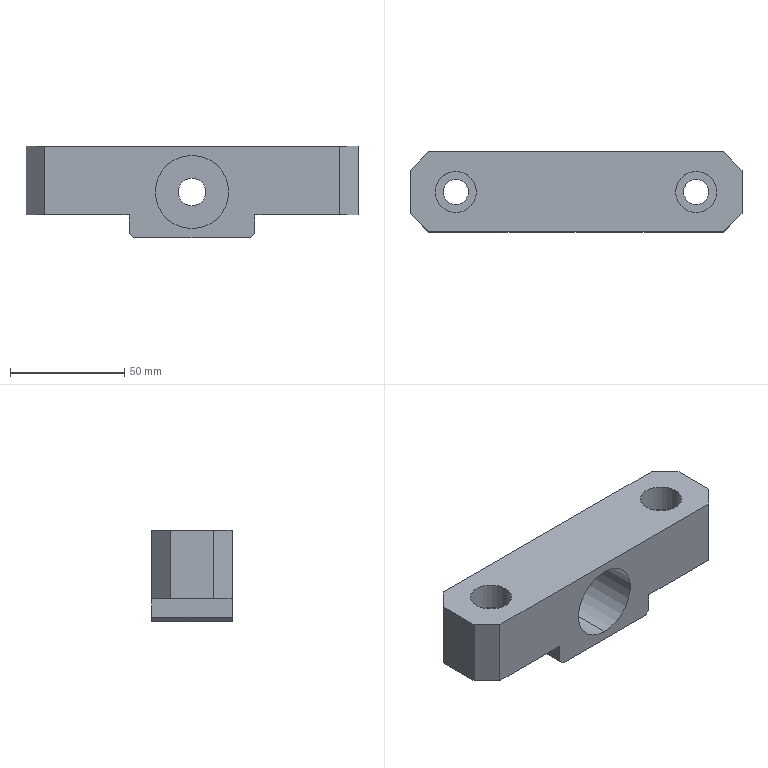Part | STEP file | LM-05-1255B_default | 1 solid | 37 faces | box 145 x 35 x 40 mm | volume 134466 mm3 | plane 21 | cylinder 16 | commonest cylinder face diameters 11 x4 18 x4 30 x4 12 x2 32 x2